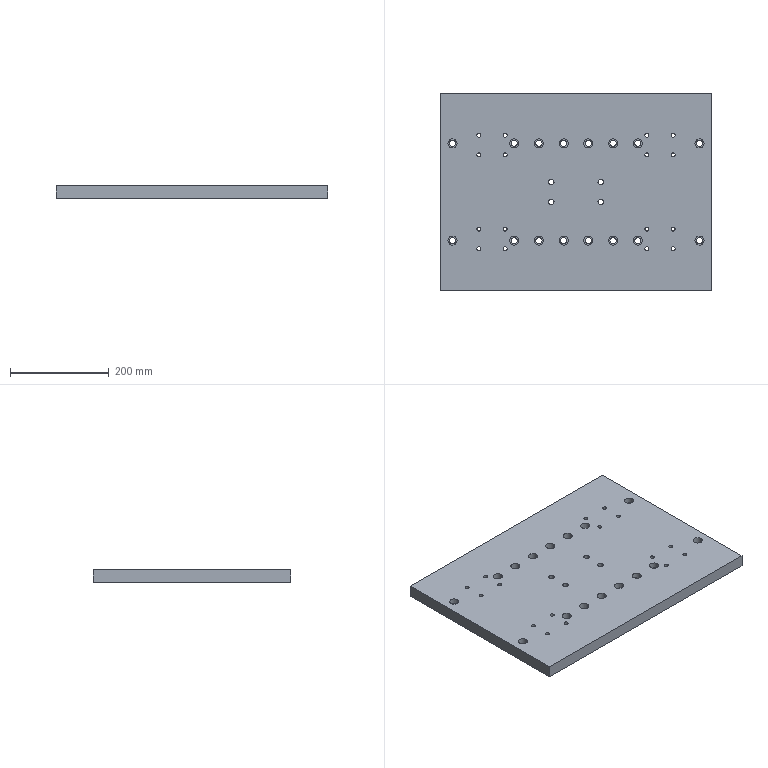Part | SolidWorks | features BaseBody 1 | 1 solid | 186 faces | box 550 x 400 x 25 mm | volume 5373061 mm3 | cylinder 144 | plane 42 | commonest cylinder face diameters 8.2 x32 12.5 x32 13.5 x32 18.5 x32 11 x8 21.48 x8